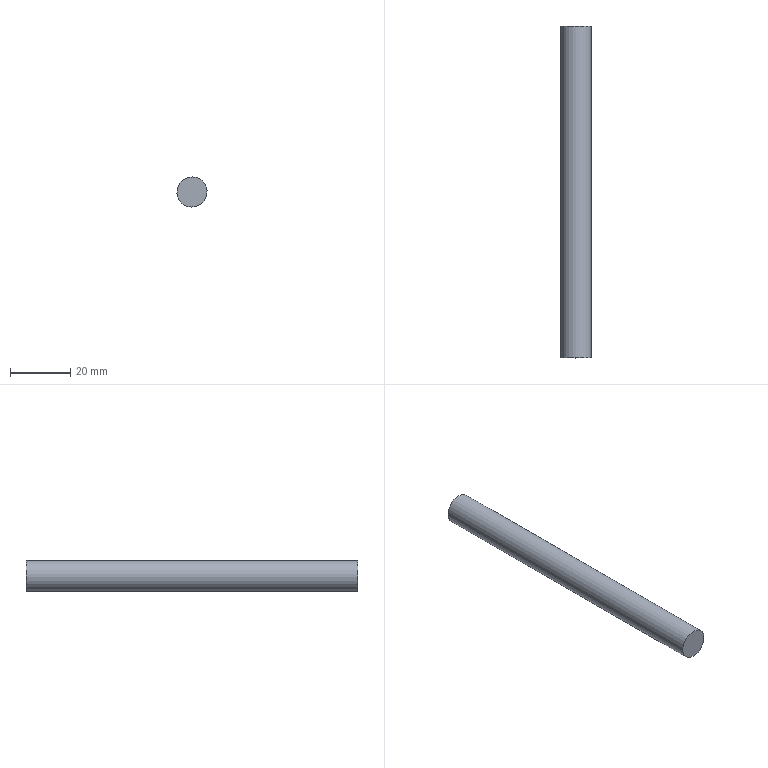Part | STEP file | solid 30 | 1 solid | 3 faces | box 10 x 110 x 10 mm | volume 8639 mm3 | plane 2 | cylinder 1 | commonest cylinder face diameters 10 x1